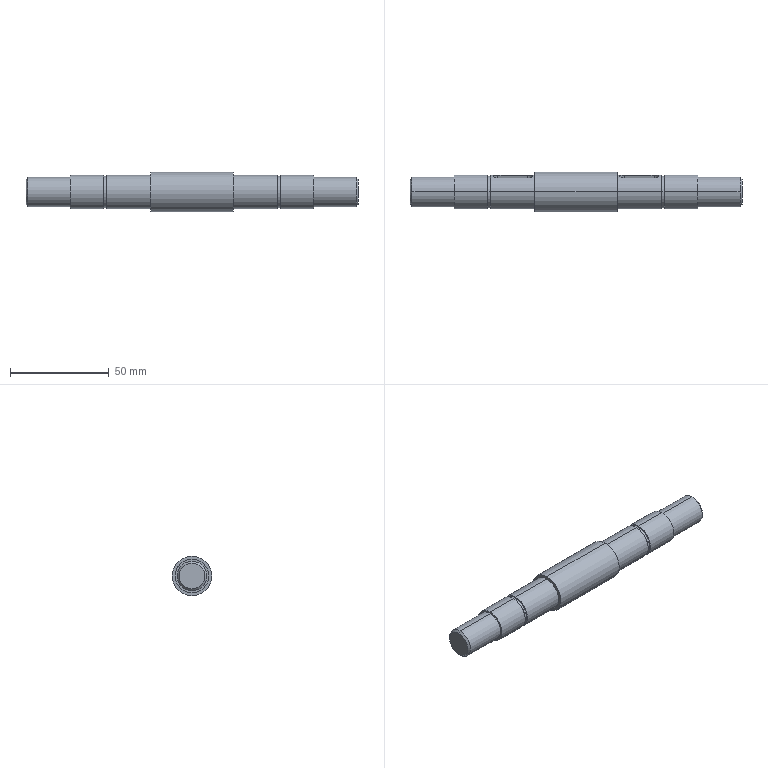Part | SolidWorks | features BaseBody 1 | 1 solid | 50 faces | box 168 x 20 x 20 mm | volume 38842 mm3 | cylinder 22 | plane 16 | spline 8 | cone 4 | commonest cylinder face diameters 17 x8 5 x4 15 x4 16 x4 20 x2